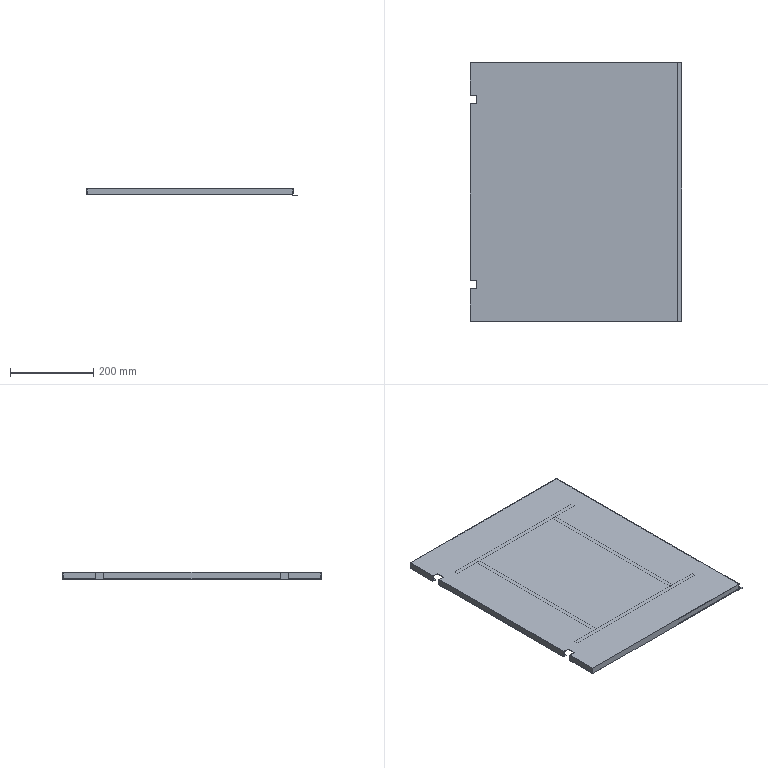Part | STEP file | 5 solids | 66 faces | box 508 x 622 x 18 mm | volume 582197 mm3 | plane 66